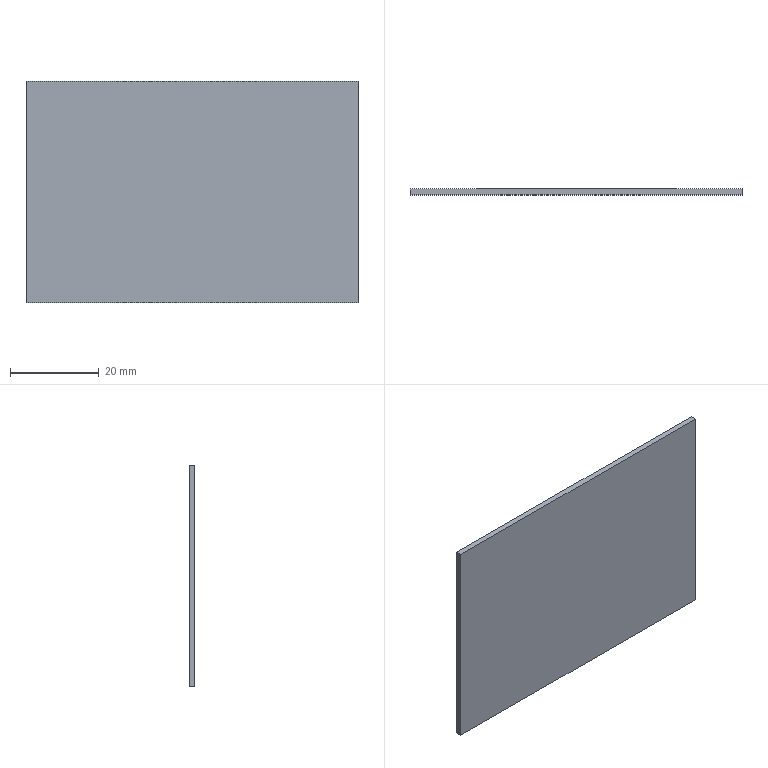Part | STEP file | Mount electronic clip cleaning part 20141015 | 1 solid | 228 faces | box 75 x 1.3 x 50 mm | volume 4576 mm3 | plane 160 | spline 68